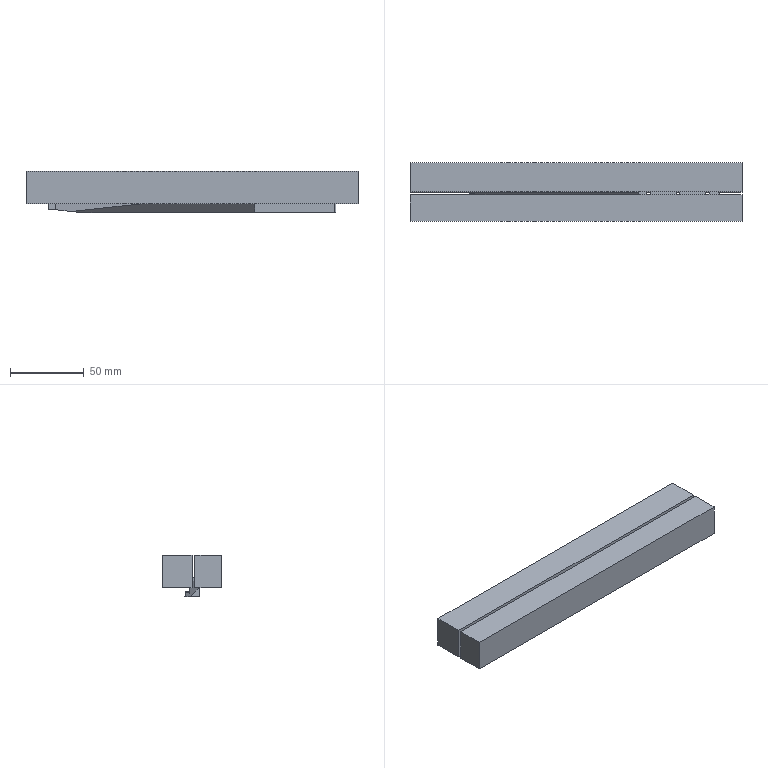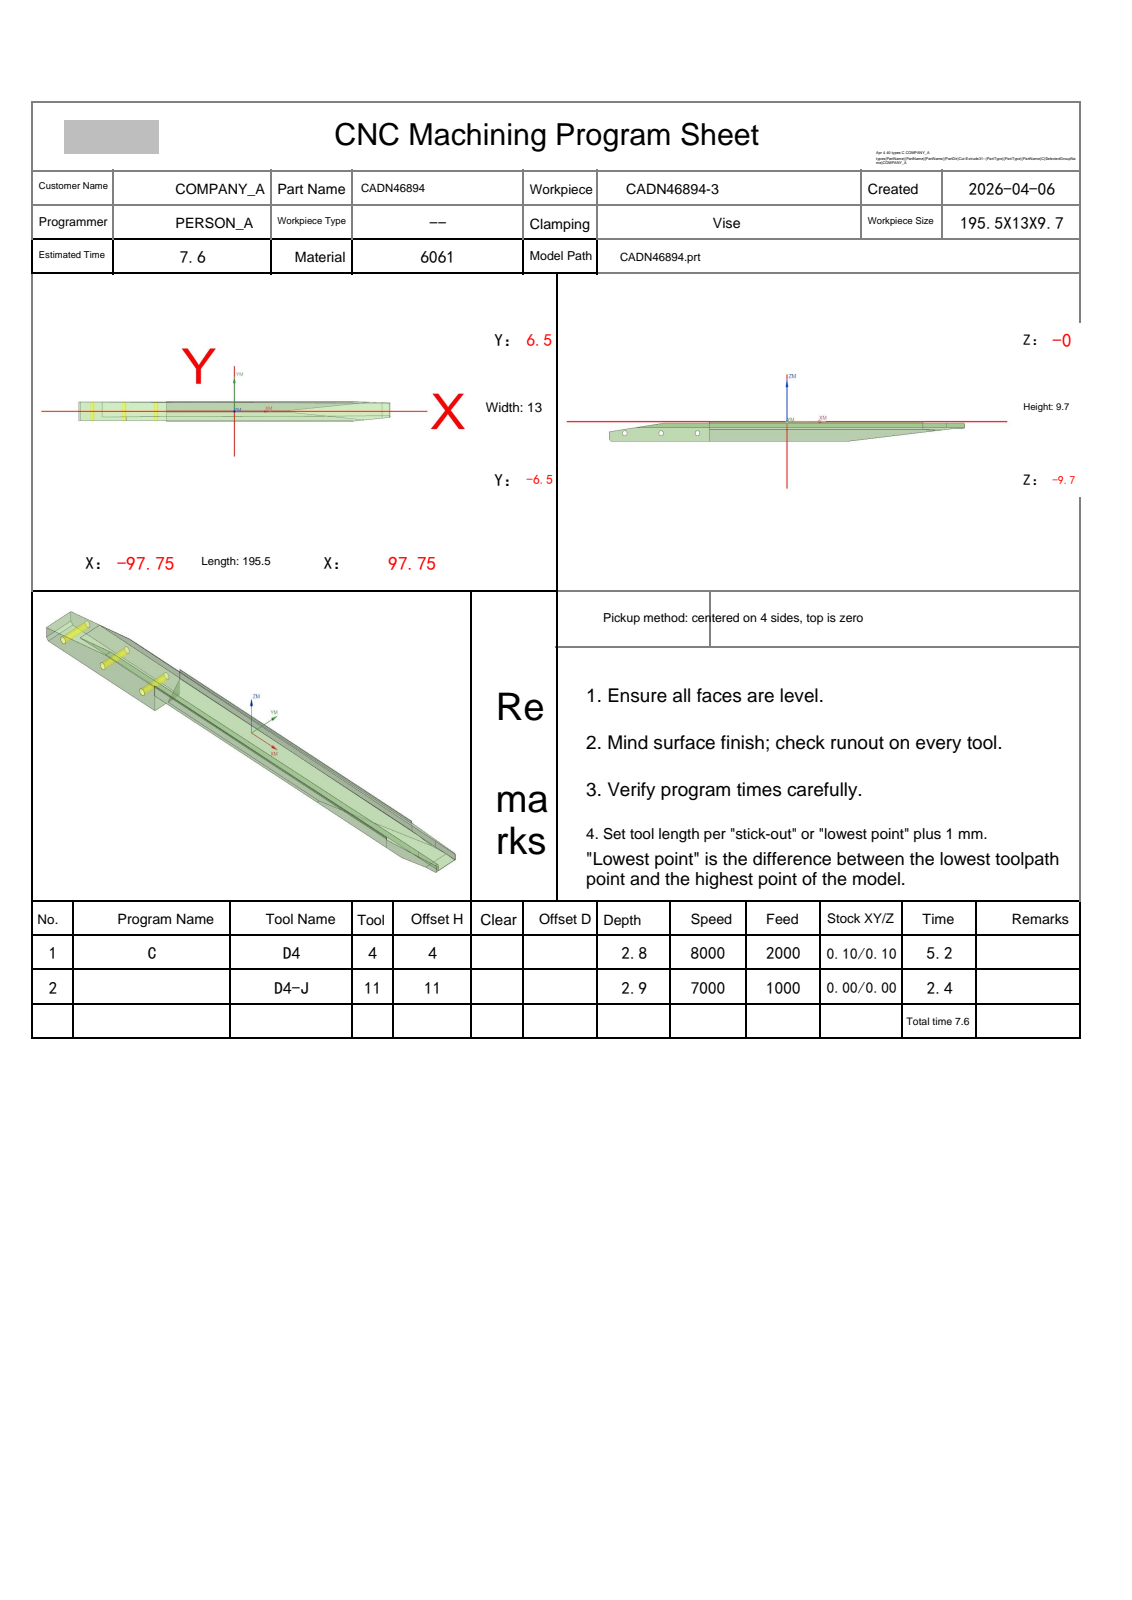NC program | NX | posted by the shop | part box 225.5 x 39.7 x 28 mm
Lines 1335 to 2406 of 20119:
N2 T17 M06
(D2-J  D=2. R=0. H=17 ce=0.00 di=0.00)
G00 G90 G54 X-18.314 Y-3.537 M03 S8000
G43 H17 Z44.
M08
Z-5.9
G01 X-18.313 Y-3.54 Z-5.93 F800.
X-18.309 Y-3.547 Z-5.958
X-18.302 Y-3.557 Z-5.982
X-18.293 Y-3.57 Z-6.004
X-18.282 Y-3.586 Z-6.023
X-18.268 Y-3.603 Z-6.04
X-18.253 Y-3.621 Z-6.054
X-18.235 Y-3.639 Z-6.066
X-18.215 Y-3.657 Z-6.076
X-18.193 Y-3.673 Z-6.084
X-18.169 Y-3.687 Z-6.09
X-18.143 Y-3.699 Z-6.095
X-18.115 Y-3.707 Z-6.098
X-18.086 Y-3.711 Z-6.099
X-18.055 Y-3.71 Z-6.1
X-5.108 Y-2.306
X-5. Y-2.3
X-3.
G02 X-.827 Y-2.797 I0.0 J-5.
X-1. Y-2.205 I.927 J.592
G01 Y-1.795
G02 X-.827 Y-1.203 I1.1 J0.0
G01 X-.847 Y-1.213
G02 X-3. Y-1.7 I-2.153 J4.513
G01 X-18.163
X-18.203 Y-1.718 Z-6.101
X-18.236 Y-1.767 Z-6.103
X-18.263 Y-1.843 Z-6.106
X-18.285 Y-1.939 Z-6.11
X-18.303 Y-2.05 Z-6.115
X-18.316 Y-2.17 Z-6.121
X-18.325 Y-2.293 Z-6.127
X-18.334 Y-2.578 Z-6.142
X-18.322 Y-2.858 Z-6.158
X-18.287 Y-3.14 Z-6.173
X-18.265 Y-3.262 Z-6.179
X-18.238 Y-3.379 Z-6.185
X-18.207 Y-3.487 Z-6.19
X-18.173 Y-3.58 Z-6.194
X-18.136 Y-3.652 Z-6.197
X-18.096 Y-3.697 Z-6.199
X-18.055 Y-3.71 Z-6.2
X-5.108 Y-2.306
X-5. Y-2.3
X-3.
G02 X-.827 Y-2.797 I0.0 J-5.
X-1. Y-2.205 I.927 J.592
G01 Y-1.795
G02 X-.827 Y-1.203 I1.1 J0.0
G01 X-.847 Y-1.213
G02 X-3. Y-1.7 I-2.153 J4.513
G01 X-18.163
X-18.203 Y-1.718 Z-6.201
X-18.236 Y-1.767 Z-6.203
X-18.263 Y-1.843 Z-6.206
X-18.285 Y-1.939 Z-6.21
X-18.303 Y-2.05 Z-6.215
X-18.316 Y-2.17 Z-6.221
X-18.325 Y-2.293 Z-6.227
X-18.334 Y-2.578 Z-6.242
X-18.322 Y-2.858 Z-6.258
X-18.287 Y-3.14 Z-6.273
X-18.265 Y-3.262 Z-6.279
X-18.238 Y-3.379 Z-6.285
X-18.207 Y-3.487 Z-6.29
X-18.173 Y-3.58 Z-6.294
X-18.136 Y-3.652 Z-6.297
X-18.096 Y-3.697 Z-6.299
X-18.055 Y-3.71 Z-6.3
X-5.108 Y-2.306
X-5. Y-2.3
X-3.
G02 X-.827 Y-2.797 I0.0 J-5.
X-1. Y-2.205 I.927 J.592
G01 Y-1.795
G02 X-.827 Y-1.203 I1.1 J0.0
G01 X-.847 Y-1.213
G02 X-3. Y-1.7 I-2.153 J4.513
G01 X-18.163
X-18.203 Y-1.718 Z-6.301
X-18.236 Y-1.767 Z-6.303
X-18.263 Y-1.843 Z-6.306
X-18.285 Y-1.939 Z-6.31
X-18.303 Y-2.05 Z-6.315
X-18.316 Y-2.17 Z-6.321
X-18.325 Y-2.293 Z-6.327
X-18.334 Y-2.578 Z-6.342
X-18.322 Y-2.858 Z-6.358
X-18.287 Y-3.14 Z-6.373
X-18.265 Y-3.262 Z-6.379
X-18.238 Y-3.379 Z-6.385
X-18.207 Y-3.487 Z-6.39
X-18.173 Y-3.58 Z-6.394
X-18.136 Y-3.652 Z-6.397
X-18.096 Y-3.697 Z-6.399
X-18.055 Y-3.71 Z-6.4
X-5.108 Y-2.306
X-5. Y-2.3
X-3.
G02 X-.827 Y-2.797 I0.0 J-5.
X-1. Y-2.205 I.927 J.592
G01 Y-1.795
G02 X-.827 Y-1.203 I1.1 J0.0
G01 X-.847 Y-1.213
G02 X-3. Y-1.7 I-2.153 J4.513
G01 X-18.163
X-18.203 Y-1.718 Z-6.401
X-18.236 Y-1.767 Z-6.403
X-18.263 Y-1.843 Z-6.406
X-18.285 Y-1.939 Z-6.41
X-18.303 Y-2.05 Z-6.415
X-18.316 Y-2.17 Z-6.421
X-18.325 Y-2.293 Z-6.427
X-18.334 Y-2.578 Z-6.442
X-18.322 Y-2.858 Z-6.458
X-18.287 Y-3.14 Z-6.473
X-18.265 Y-3.262 Z-6.479
X-18.238 Y-3.379 Z-6.485
X-18.207 Y-3.487 Z-6.49
X-18.173 Y-3.58 Z-6.494
X-18.136 Y-3.652 Z-6.497
X-18.096 Y-3.697 Z-6.499
X-18.055 Y-3.71 Z-6.5
X-5.108 Y-2.306
X-5. Y-2.3
X-3.
G02 X-.827 Y-2.797 I0.0 J-5.
X-1. Y-2.205 I.927 J.592
G01 Y-1.795
G02 X-.827 Y-1.203 I1.1 J0.0
G01 X-.847 Y-1.213
G02 X-3. Y-1.7 I-2.153 J4.513
G01 X-18.163
X-18.203 Y-1.718 Z-6.501
X-18.236 Y-1.767 Z-6.503
X-18.263 Y-1.843 Z-6.506
X-18.285 Y-1.939 Z-6.51
X-18.303 Y-2.05 Z-6.515
X-18.316 Y-2.17 Z-6.521
X-18.325 Y-2.293 Z-6.527
X-18.334 Y-2.578 Z-6.542
X-18.322 Y-2.858 Z-6.558
X-18.287 Y-3.14 Z-6.573
X-18.265 Y-3.262 Z-6.579
X-18.238 Y-3.379 Z-6.585
X-18.207 Y-3.487 Z-6.59
X-18.173 Y-3.58 Z-6.594
X-18.136 Y-3.652 Z-6.597
X-18.096 Y-3.697 Z-6.599
X-18.055 Y-3.71 Z-6.6
X-5.108 Y-2.306
X-5. Y-2.3
X-3.
G02 X-.827 Y-2.797 I0.0 J-5.
X-1. Y-2.205 I.927 J.592
G01 Y-1.795
G02 X-.827 Y-1.203 I1.1 J0.0
G01 X-.847 Y-1.213
G02 X-3. Y-1.7 I-2.153 J4.513
G01 X-18.163
X-18.203 Y-1.718 Z-6.601
X-18.236 Y-1.767 Z-6.603
X-18.263 Y-1.843 Z-6.606
X-18.285 Y-1.939 Z-6.61
X-18.303 Y-2.05 Z-6.615
X-18.316 Y-2.17 Z-6.621
X-18.325 Y-2.293 Z-6.627
X-18.334 Y-2.578 Z-6.642
X-18.322 Y-2.858 Z-6.658
X-18.287 Y-3.14 Z-6.673
X-18.265 Y-3.262 Z-6.679
X-18.238 Y-3.379 Z-6.685
X-18.207 Y-3.487 Z-6.69
X-18.173 Y-3.58 Z-6.694
X-18.136 Y-3.652 Z-6.697
X-18.096 Y-3.697 Z-6.699
X-18.055 Y-3.71 Z-6.7
X-5.108 Y-2.306
X-5. Y-2.3
X-3.
G02 X-.827 Y-2.797 I0.0 J-5.
X-1. Y-2.205 I.927 J.592
G01 Y-1.795
G02 X-.827 Y-1.203 I1.1 J0.0
G01 X-.847 Y-1.213
G02 X-3. Y-1.7 I-2.153 J4.513
G01 X-18.163
X-18.203 Y-1.718 Z-6.701
X-18.236 Y-1.767 Z-6.703
X-18.263 Y-1.843 Z-6.706
X-18.285 Y-1.939 Z-6.71
X-18.303 Y-2.05 Z-6.715
X-18.316 Y-2.17 Z-6.721
X-18.325 Y-2.293 Z-6.727
X-18.334 Y-2.578 Z-6.742
X-18.322 Y-2.858 Z-6.758
X-18.287 Y-3.14 Z-6.773
X-18.265 Y-3.262 Z-6.779
X-18.238 Y-3.379 Z-6.785
X-18.207 Y-3.487 Z-6.79
X-18.173 Y-3.58 Z-6.794
X-18.136 Y-3.652 Z-6.797
X-18.096 Y-3.697 Z-6.799
X-18.055 Y-3.71 Z-6.8
X-5.108 Y-2.306
X-5. Y-2.3
X-3.
G02 X-.827 Y-2.797 I0.0 J-5.
X-1. Y-2.205 I.927 J.592
G01 Y-1.795
G02 X-.827 Y-1.203 I1.1 J0.0
G01 X-.847 Y-1.213
G02 X-3. Y-1.7 I-2.153 J4.513
G01 X-18.163
X-18.203 Y-1.718 Z-6.801
X-18.236 Y-1.767 Z-6.803
X-18.263 Y-1.843 Z-6.806
X-18.285 Y-1.939 Z-6.81
X-18.303 Y-2.05 Z-6.815
X-18.316 Y-2.17 Z-6.821
X-18.325 Y-2.293 Z-6.827
X-18.334 Y-2.578 Z-6.842
X-18.322 Y-2.858 Z-6.858
X-18.287 Y-3.14 Z-6.873
X-18.265 Y-3.262 Z-6.879
X-18.238 Y-3.379 Z-6.885
X-18.207 Y-3.487 Z-6.89
X-18.173 Y-3.58 Z-6.894
X-18.136 Y-3.652 Z-6.897
X-18.096 Y-3.697 Z-6.899
X-18.055 Y-3.71 Z-6.9
X-5.108 Y-2.306
X-5. Y-2.3
X-3.
G02 X-.827 Y-2.797 I0.0 J-5.
X-1. Y-2.205 I.927 J.592
G01 Y-1.795
G02 X-.827 Y-1.203 I1.1 J0.0
G01 X-.847 Y-1.213
G02 X-3. Y-1.7 I-2.153 J4.513
G01 X-18.163
X-18.203 Y-1.718 Z-6.901
X-18.236 Y-1.767 Z-6.903
X-18.263 Y-1.843 Z-6.906
X-18.285 Y-1.939 Z-6.91
X-18.303 Y-2.05 Z-6.915
X-18.316 Y-2.17 Z-6.921
X-18.325 Y-2.293 Z-6.927
X-18.334 Y-2.578 Z-6.942
X-18.322 Y-2.858 Z-6.958
X-18.287 Y-3.14 Z-6.973
X-18.265 Y-3.262 Z-6.979
X-18.238 Y-3.379 Z-6.985
X-18.207 Y-3.487 Z-6.99
X-18.173 Y-3.58 Z-6.994
X-18.136 Y-3.652 Z-6.997
X-18.096 Y-3.697 Z-6.999
X-18.055 Y-3.71 Z-7.
X-5.108 Y-2.306
X-5. Y-2.3
X-3.
G02 X-.827 Y-2.797 I0.0 J-5.
X-1. Y-2.205 I.927 J.592
G01 Y-1.795
G02 X-.827 Y-1.203 I1.1 J0.0
G01 X-.847 Y-1.213
G02 X-3. Y-1.7 I-2.153 J4.513
G01 X-18.163
X-18.203 Y-1.718 Z-7.001
X-18.236 Y-1.767 Z-7.003
X-18.263 Y-1.843 Z-7.006
X-18.285 Y-1.939 Z-7.01
X-18.303 Y-2.05 Z-7.015
X-18.316 Y-2.17 Z-7.021
X-18.325 Y-2.293 Z-7.027
X-18.334 Y-2.578 Z-7.042
X-18.322 Y-2.858 Z-7.058
X-18.287 Y-3.14 Z-7.073
X-18.265 Y-3.262 Z-7.079
X-18.238 Y-3.379 Z-7.085
X-18.207 Y-3.487 Z-7.09
X-18.173 Y-3.58 Z-7.094
X-18.136 Y-3.652 Z-7.097
X-18.096 Y-3.697 Z-7.099
X-18.055 Y-3.71 Z-7.1
X-5.108 Y-2.306
X-5. Y-2.3
X-3.
G02 X-.827 Y-2.797 I0.0 J-5.
X-1. Y-2.205 I.927 J.592
G01 Y-1.795
G02 X-.827 Y-1.203 I1.1 J0.0
G01 X-.847 Y-1.213
G02 X-3. Y-1.7 I-2.153 J4.513
G01 X-18.163
X-18.203 Y-1.718 Z-7.101
X-18.236 Y-1.767 Z-7.103
X-18.263 Y-1.843 Z-7.106
X-18.285 Y-1.939 Z-7.11
X-18.303 Y-2.05 Z-7.115
X-18.316 Y-2.17 Z-7.121
X-18.325 Y-2.293 Z-7.127
X-18.334 Y-2.578 Z-7.142
X-18.322 Y-2.858 Z-7.158
X-18.287 Y-3.14 Z-7.173
X-18.265 Y-3.262 Z-7.179
X-18.238 Y-3.379 Z-7.185
X-18.207 Y-3.487 Z-7.19
X-18.173 Y-3.58 Z-7.194
X-18.136 Y-3.652 Z-7.197
X-18.096 Y-3.697 Z-7.199
X-18.055 Y-3.71 Z-7.2
X-5.108 Y-2.306
X-5. Y-2.3
X-3.
G02 X-.827 Y-2.797 I0.0 J-5.
X-1. Y-2.205 I.927 J.592
G01 Y-1.795
G02 X-.827 Y-1.203 I1.1 J0.0
G01 X-.847 Y-1.213
G02 X-3. Y-1.7 I-2.153 J4.513
G01 X-18.163
X-18.203 Y-1.718 Z-7.201
X-18.236 Y-1.767 Z-7.203
X-18.263 Y-1.843 Z-7.206
X-18.285 Y-1.939 Z-7.21
X-18.303 Y-2.05 Z-7.215
X-18.316 Y-2.17 Z-7.221
X-18.325 Y-2.293 Z-7.227
X-18.334 Y-2.578 Z-7.242
X-18.322 Y-2.858 Z-7.258
X-18.287 Y-3.14 Z-7.273
X-18.265 Y-3.262 Z-7.279
X-18.238 Y-3.379 Z-7.285
X-18.207 Y-3.487 Z-7.29
X-18.173 Y-3.58 Z-7.294
X-18.136 Y-3.652 Z-7.297
X-18.096 Y-3.697 Z-7.299
X-18.055 Y-3.71 Z-7.3
X-5.108 Y-2.306
X-5. Y-2.3
X-3.
G02 X-.827 Y-2.797 I0.0 J-5.
X-1. Y-2.205 I.927 J.592
G01 Y-1.795
G02 X-.827 Y-1.203 I1.1 J0.0
G01 X-.847 Y-1.213
G02 X-3. Y-1.7 I-2.153 J4.513
G01 X-18.163
X-18.203 Y-1.718 Z-7.301
X-18.236 Y-1.767 Z-7.303
X-18.263 Y-1.843 Z-7.306
X-18.285 Y-1.939 Z-7.31
X-18.303 Y-2.05 Z-7.315
X-18.316 Y-2.17 Z-7.321
X-18.325 Y-2.293 Z-7.327
X-18.334 Y-2.578 Z-7.342
X-18.322 Y-2.858 Z-7.358
X-18.287 Y-3.14 Z-7.373
X-18.265 Y-3.262 Z-7.379
X-18.238 Y-3.379 Z-7.385
X-18.207 Y-3.487 Z-7.39
X-18.173 Y-3.58 Z-7.394
X-18.136 Y-3.652 Z-7.397
X-18.096 Y-3.697 Z-7.399
X-18.055 Y-3.71 Z-7.4
X-5.108 Y-2.306
X-5. Y-2.3
X-3.
G02 X-.827 Y-2.797 I0.0 J-5.
X-1. Y-2.205 I.927 J.592
G01 Y-1.795
G02 X-.827 Y-1.203 I1.1 J0.0
G01 X-.847 Y-1.213
G02 X-3. Y-1.7 I-2.153 J4.513
G01 X-18.163
X-18.203 Y-1.718 Z-7.401
X-18.236 Y-1.767 Z-7.403
X-18.263 Y-1.843 Z-7.406
X-18.285 Y-1.939 Z-7.41
X-18.303 Y-2.05 Z-7.415
X-18.316 Y-2.17 Z-7.421
X-18.325 Y-2.293 Z-7.427
X-18.334 Y-2.578 Z-7.442
X-18.322 Y-2.858 Z-7.458
X-18.287 Y-3.14 Z-7.473
X-18.265 Y-3.262 Z-7.479
X-18.238 Y-3.379 Z-7.485
X-18.207 Y-3.487 Z-7.49
X-18.173 Y-3.58 Z-7.494
X-18.136 Y-3.652 Z-7.497
X-18.096 Y-3.697 Z-7.499
X-18.055 Y-3.71 Z-7.5
X-5.108 Y-2.306
X-5. Y-2.3
X-3.
G02 X-.827 Y-2.797 I0.0 J-5.
X-1. Y-2.205 I.927 J.592
G01 Y-1.795
G02 X-.827 Y-1.203 I1.1 J0.0
G01 X-.847 Y-1.213
G02 X-3. Y-1.7 I-2.153 J4.513
G01 X-18.163
X-18.203 Y-1.718 Z-7.501
X-18.236 Y-1.767 Z-7.503
X-18.263 Y-1.843 Z-7.506
X-18.285 Y-1.939 Z-7.51
X-18.303 Y-2.05 Z-7.515
X-18.316 Y-2.17 Z-7.521
X-18.325 Y-2.293 Z-7.527
X-18.334 Y-2.578 Z-7.542
X-18.322 Y-2.858 Z-7.558
X-18.287 Y-3.14 Z-7.573
X-18.265 Y-3.262 Z-7.579
X-18.238 Y-3.379 Z-7.585
X-18.207 Y-3.487 Z-7.59
X-18.173 Y-3.58 Z-7.594
X-18.136 Y-3.652 Z-7.597
X-18.096 Y-3.697 Z-7.599
X-18.055 Y-3.71 Z-7.6
X-5.108 Y-2.306
X-5. Y-2.3
X-3.
G02 X-.827 Y-2.797 I0.0 J-5.
X-1. Y-2.205 I.927 J.592
G01 Y-1.795
G02 X-.827 Y-1.203 I1.1 J0.0
G01 X-.847 Y-1.213
G02 X-3. Y-1.7 I-2.153 J4.513
G01 X-18.163
X-18.203 Y-1.718 Z-7.601
X-18.236 Y-1.767 Z-7.603
X-18.263 Y-1.843 Z-7.606
X-18.285 Y-1.939 Z-7.61
X-18.303 Y-2.05 Z-7.615
X-18.316 Y-2.17 Z-7.621
X-18.325 Y-2.293 Z-7.627
X-18.334 Y-2.578 Z-7.642
X-18.322 Y-2.858 Z-7.658
X-18.287 Y-3.14 Z-7.673
X-18.265 Y-3.262 Z-7.679
X-18.238 Y-3.379 Z-7.685
X-18.207 Y-3.487 Z-7.69
X-18.173 Y-3.58 Z-7.694
X-18.136 Y-3.652 Z-7.697
X-18.096 Y-3.697 Z-7.699
X-18.055 Y-3.71 Z-7.7
X-5.108 Y-2.306
X-5. Y-2.3
X-3.
G02 X-.827 Y-2.797 I0.0 J-5.
X-1. Y-2.205 I.927 J.592
G01 Y-1.795
G02 X-.827 Y-1.203 I1.1 J0.0
G01 X-.847 Y-1.213
G02 X-3. Y-1.7 I-2.153 J4.513
G01 X-18.163
X-18.203 Y-1.718 Z-7.701
X-18.236 Y-1.767 Z-7.703
X-18.263 Y-1.843 Z-7.706
X-18.285 Y-1.939 Z-7.71
X-18.303 Y-2.05 Z-7.715
X-18.316 Y-2.17 Z-7.721
X-18.325 Y-2.293 Z-7.727
X-18.334 Y-2.578 Z-7.742
X-18.322 Y-2.858 Z-7.758
X-18.287 Y-3.14 Z-7.773
X-18.265 Y-3.262 Z-7.779
X-18.238 Y-3.379 Z-7.785
X-18.207 Y-3.487 Z-7.79
X-18.173 Y-3.58 Z-7.794
X-18.136 Y-3.652 Z-7.797
X-18.096 Y-3.697 Z-7.799
X-18.055 Y-3.71 Z-7.8
X-5.108 Y-2.306
X-5. Y-2.3
X-3.
G02 X-.827 Y-2.797 I0.0 J-5.
X-1. Y-2.205 I.927 J.592
G01 Y-1.795
G02 X-.827 Y-1.203 I1.1 J0.0
G01 X-.847 Y-1.213
G02 X-3. Y-1.7 I-2.153 J4.513
G01 X-18.163
X-18.203 Y-1.718 Z-7.801
X-18.236 Y-1.767 Z-7.803
X-18.263 Y-1.843 Z-7.806
X-18.285 Y-1.939 Z-7.81
X-18.303 Y-2.05 Z-7.815
X-18.316 Y-2.17 Z-7.821
X-18.325 Y-2.293 Z-7.827
X-18.334 Y-2.578 Z-7.842
X-18.322 Y-2.858 Z-7.858
X-18.287 Y-3.14 Z-7.873
X-18.265 Y-3.262 Z-7.879
X-18.238 Y-3.379 Z-7.885
X-18.207 Y-3.487 Z-7.89
X-18.173 Y-3.58 Z-7.894
X-18.136 Y-3.652 Z-7.897
X-18.096 Y-3.697 Z-7.899
X-18.055 Y-3.71 Z-7.9
X-5.108 Y-2.306
X-5. Y-2.3
X-3.
G02 X-.827 Y-2.797 I0.0 J-5.
X-1. Y-2.205 I.927 J.592
G01 Y-1.795
G02 X-.827 Y-1.203 I1.1 J0.0
G01 X-.847 Y-1.213
G02 X-3. Y-1.7 I-2.153 J4.513
G01 X-18.163
X-18.203 Y-1.718 Z-7.901
X-18.236 Y-1.767 Z-7.903
X-18.263 Y-1.843 Z-7.906
X-18.285 Y-1.939 Z-7.91
X-18.303 Y-2.05 Z-7.915
X-18.316 Y-2.17 Z-7.921
X-18.325 Y-2.293 Z-7.927
X-18.334 Y-2.578 Z-7.942
X-18.322 Y-2.858 Z-7.958
X-18.287 Y-3.14 Z-7.973
X-18.265 Y-3.262 Z-7.979
X-18.238 Y-3.379 Z-7.985
X-18.207 Y-3.487 Z-7.99
X-18.173 Y-3.58 Z-7.994
X-18.136 Y-3.652 Z-7.997
X-18.096 Y-3.697 Z-7.999
X-18.055 Y-3.71 Z-8.
X-5.108 Y-2.306
X-5. Y-2.3
X-3.
G02 X-.827 Y-2.797 I0.0 J-5.
X-1. Y-2.205 I.927 J.592
G01 Y-1.795
G02 X-.827 Y-1.203 I1.1 J0.0
G01 X-.847 Y-1.213
G02 X-3. Y-1.7 I-2.153 J4.513
G01 X-18.163
X-18.203 Y-1.718 Z-8.001
X-18.236 Y-1.767 Z-8.003
X-18.263 Y-1.843 Z-8.006
X-18.285 Y-1.939 Z-8.01
X-18.303 Y-2.05 Z-8.015
X-18.316 Y-2.17 Z-8.021
X-18.325 Y-2.293 Z-8.027
X-18.334 Y-2.578 Z-8.042
X-18.322 Y-2.858 Z-8.058
X-18.287 Y-3.14 Z-8.073
X-18.265 Y-3.262 Z-8.079
X-18.238 Y-3.379 Z-8.085
X-18.207 Y-3.487 Z-8.09
X-18.173 Y-3.58 Z-8.094
X-18.136 Y-3.652 Z-8.097
X-18.096 Y-3.697 Z-8.099
X-18.055 Y-3.71 Z-8.1
X-5.108 Y-2.306
X-5. Y-2.3
X-3.
G02 X-.827 Y-2.797 I0.0 J-5.
X-1. Y-2.205 I.927 J.592
G01 Y-1.795
G02 X-.827 Y-1.203 I1.1 J0.0
G01 X-.847 Y-1.213
G02 X-3. Y-1.7 I-2.153 J4.513
G01 X-18.163
X-18.203 Y-1.718 Z-8.101
X-18.236 Y-1.767 Z-8.103
X-18.263 Y-1.843 Z-8.106
X-18.285 Y-1.939 Z-8.11
X-18.303 Y-2.05 Z-8.115
X-18.316 Y-2.17 Z-8.121
X-18.325 Y-2.293 Z-8.127
X-18.334 Y-2.578 Z-8.142
X-18.322 Y-2.858 Z-8.158
X-18.287 Y-3.14 Z-8.173
X-18.265 Y-3.262 Z-8.179
X-18.238 Y-3.379 Z-8.185
X-18.207 Y-3.487 Z-8.19
X-18.173 Y-3.58 Z-8.194
X-18.136 Y-3.652 Z-8.197
X-18.096 Y-3.697 Z-8.199
X-18.055 Y-3.71 Z-8.2
X-5.108 Y-2.306
X-5. Y-2.3
X-3.
G02 X-.827 Y-2.797 I0.0 J-5.
X-1. Y-2.205 I.927 J.592
G01 Y-1.795
G02 X-.827 Y-1.203 I1.1 J0.0
G01 X-.847 Y-1.213
G02 X-3. Y-1.7 I-2.153 J4.513
G01 X-18.163
X-18.203 Y-1.718 Z-8.201
X-18.236 Y-1.767 Z-8.203
X-18.263 Y-1.843 Z-8.206
X-18.285 Y-1.939 Z-8.21
X-18.303 Y-2.05 Z-8.215
X-18.316 Y-2.17 Z-8.221
X-18.325 Y-2.293 Z-8.227
X-18.334 Y-2.578 Z-8.242
X-18.322 Y-2.858 Z-8.258
X-18.287 Y-3.14 Z-8.273
X-18.265 Y-3.262 Z-8.279
X-18.238 Y-3.379 Z-8.285
X-18.207 Y-3.487 Z-8.29
X-18.173 Y-3.58 Z-8.294
X-18.136 Y-3.652 Z-8.297
X-18.096 Y-3.697 Z-8.299
X-18.055 Y-3.71 Z-8.3
X-5.108 Y-2.306
X-5. Y-2.3
X-3.
G02 X-.827 Y-2.797 I0.0 J-5.
X-1. Y-2.205 I.927 J.592
G01 Y-1.795
G02 X-.827 Y-1.203 I1.1 J0.0
G01 X-.847 Y-1.213
G02 X-3. Y-1.7 I-2.153 J4.513
G01 X-18.163
X-18.203 Y-1.718 Z-8.301
X-18.236 Y-1.767 Z-8.303
X-18.263 Y-1.843 Z-8.306
X-18.285 Y-1.939 Z-8.31
X-18.303 Y-2.05 Z-8.315
X-18.316 Y-2.17 Z-8.321
X-18.325 Y-2.293 Z-8.327
X-18.334 Y-2.578 Z-8.342
X-18.322 Y-2.858 Z-8.358
X-18.287 Y-3.14 Z-8.373
X-18.265 Y-3.262 Z-8.379
X-18.238 Y-3.379 Z-8.385
X-18.207 Y-3.487 Z-8.39
X-18.173 Y-3.58 Z-8.394
X-18.136 Y-3.652 Z-8.397
X-18.096 Y-3.697 Z-8.399
X-18.055 Y-3.71 Z-8.4
X-5.108 Y-2.306
X-5. Y-2.3
X-3.
G02 X-.827 Y-2.797 I0.0 J-5.
X-1. Y-2.205 I.927 J.592
G01 Y-1.795
G02 X-.827 Y-1.203 I1.1 J0.0
G01 X-.847 Y-1.213
G02 X-3. Y-1.7 I-2.153 J4.513
G01 X-18.163
X-18.203 Y-1.718 Z-8.401
X-18.236 Y-1.767 Z-8.403
X-18.263 Y-1.843 Z-8.406
X-18.285 Y-1.939 Z-8.41
X-18.303 Y-2.05 Z-8.415
X-18.316 Y-2.17 Z-8.421
X-18.325 Y-2.293 Z-8.427
X-18.334 Y-2.578 Z-8.442
X-18.322 Y-2.858 Z-8.458
X-18.287 Y-3.14 Z-8.473
X-18.265 Y-3.262 Z-8.479
X-18.238 Y-3.379 Z-8.485
X-18.207 Y-3.487 Z-8.49
X-18.173 Y-3.58 Z-8.494
X-18.136 Y-3.652 Z-8.497
X-18.096 Y-3.697 Z-8.499
X-18.055 Y-3.71 Z-8.5
X-5.108 Y-2.306
X-5. Y-2.3
X-3.
G02 X-.827 Y-2.797 I0.0 J-5.
X-1. Y-2.205 I.927 J.592
G01 Y-1.795
G02 X-.827 Y-1.203 I1.1 J0.0
G01 X-.847 Y-1.213
G02 X-3. Y-1.7 I-2.153 J4.513
G01 X-18.163
X-18.203 Y-1.718 Z-8.501
X-18.236 Y-1.767 Z-8.503
X-18.263 Y-1.843 Z-8.506
X-18.285 Y-1.939 Z-8.51
X-18.303 Y-2.05 Z-8.515
X-18.316 Y-2.17 Z-8.521
X-18.325 Y-2.293 Z-8.527
X-18.334 Y-2.578 Z-8.542
X-18.322 Y-2.858 Z-8.558
X-18.287 Y-3.14 Z-8.573
X-18.265 Y-3.262 Z-8.579
X-18.238 Y-3.379 Z-8.585
X-18.207 Y-3.487 Z-8.59
X-18.173 Y-3.58 Z-8.594
X-18.136 Y-3.652 Z-8.597
X-18.096 Y-3.697 Z-8.599
X-18.055 Y-3.71 Z-8.6
X-5.108 Y-2.306
X-5. Y-2.3
X-3.
G02 X-.827 Y-2.797 I0.0 J-5.
X-1. Y-2.205 I.927 J.592
G01 Y-1.795
G02 X-.827 Y-1.203 I1.1 J0.0
G01 X-.847 Y-1.213
G02 X-3. Y-1.7 I-2.153 J4.513
G01 X-18.163
X-18.203 Y-1.718 Z-8.601
X-18.236 Y-1.767 Z-8.603
X-18.263 Y-1.843 Z-8.606
X-18.285 Y-1.939 Z-8.61
X-18.303 Y-2.05 Z-8.615
X-18.316 Y-2.17 Z-8.621
X-18.325 Y-2.293 Z-8.627
X-18.334 Y-2.578 Z-8.642
X-18.322 Y-2.858 Z-8.658
X-18.287 Y-3.14 Z-8.673
X-18.265 Y-3.262 Z-8.679
X-18.238 Y-3.379 Z-8.685
X-18.207 Y-3.487 Z-8.69
X-18.173 Y-3.58 Z-8.694
X-18.136 Y-3.652 Z-8.697
X-18.096 Y-3.697 Z-8.699
X-18.055 Y-3.71 Z-8.7
X-5.108 Y-2.306
X-5. Y-2.3
X-3.
G02 X-.827 Y-2.797 I0.0 J-5.
X-1. Y-2.205 I.927 J.592
G01 Y-1.795
G02 X-.827 Y-1.203 I1.1 J0.0
G01 X-.847 Y-1.213
G02 X-3. Y-1.7 I-2.153 J4.513
G01 X-18.163
X-18.203 Y-1.718 Z-8.701
X-18.236 Y-1.767 Z-8.703
X-18.263 Y-1.843 Z-8.706
X-18.285 Y-1.939 Z-8.71
X-18.303 Y-2.05 Z-8.715
X-18.316 Y-2.17 Z-8.721
X-18.325 Y-2.293 Z-8.727
X-18.334 Y-2.578 Z-8.742
X-18.322 Y-2.858 Z-8.758
X-18.287 Y-3.14 Z-8.773
X-18.265 Y-3.262 Z-8.779
X-18.238 Y-3.379 Z-8.785
X-18.207 Y-3.487 Z-8.79
X-18.173 Y-3.58 Z-8.794
X-18.136 Y-3.652 Z-8.797
X-18.096 Y-3.697 Z-8.799
X-18.055 Y-3.71 Z-8.8
X-5.108 Y-2.306
X-5. Y-2.3
X-3.
G02 X-.827 Y-2.797 I0.0 J-5.
X-1. Y-2.205 I.927 J.592
G01 Y-1.795
G02 X-.827 Y-1.203 I1.1 J0.0
G01 X-.847 Y-1.213
G02 X-3. Y-1.7 I-2.153 J4.513
G01 X-18.163
X-18.203 Y-1.718 Z-8.801
X-18.236 Y-1.767 Z-8.803
X-18.263 Y-1.843 Z-8.806
X-18.285 Y-1.939 Z-8.81
X-18.303 Y-2.05 Z-8.815
X-18.316 Y-2.17 Z-8.821
X-18.325 Y-2.293 Z-8.827
X-18.334 Y-2.578 Z-8.842
X-18.322 Y-2.858 Z-8.858
X-18.287 Y-3.14 Z-8.873
X-18.265 Y-3.262 Z-8.879
X-18.238 Y-3.379 Z-8.885
X-18.207 Y-3.487 Z-8.89
X-18.173 Y-3.58 Z-8.894
X-18.136 Y-3.652 Z-8.897
X-18.096 Y-3.697 Z-8.899
X-18.055 Y-3.71 Z-8.9
X-5.108 Y-2.306
X-5. Y-2.3
X-3.
G02 X-.827 Y-2.797 I0.0 J-5.
X-1. Y-2.205 I.927 J.592
G01 Y-1.795
G02 X-.827 Y-1.203 I1.1 J0.0
G01 X-.847 Y-1.213
G02 X-3. Y-1.7 I-2.153 J4.513
G01 X-18.163
X-18.203 Y-1.718 Z-8.901
X-18.236 Y-1.767 Z-8.903
X-18.263 Y-1.843 Z-8.906
X-18.285 Y-1.939 Z-8.91
X-18.303 Y-2.05 Z-8.915
X-18.316 Y-2.17 Z-8.921
X-18.325 Y-2.293 Z-8.927
X-18.334 Y-2.578 Z-8.942
X-18.322 Y-2.858 Z-8.958
X-18.287 Y-3.14 Z-8.973
X-18.265 Y-3.262 Z-8.979
X-18.238 Y-3.379 Z-8.985
X-18.207 Y-3.487 Z-8.99
X-18.173 Y-3.58 Z-8.994
X-18.136 Y-3.652 Z-8.997
X-18.096 Y-3.697 Z-8.999
X-18.055 Y-3.71 Z-9.
X-5.108 Y-2.306
X-5. Y-2.3
X-3.
G02 X-.827 Y-2.797 I0.0 J-5.
X-1. Y-2.205 I.927 J.592
G01 Y-1.795
G02 X-.827 Y-1.203 I1.1 J0.0
G01 X-.847 Y-1.213
G02 X-3. Y-1.7 I-2.153 J4.513
G01 X-18.163
X-18.203 Y-1.718 Z-9.001
X-18.236 Y-1.767 Z-9.003
X-18.263 Y-1.843 Z-9.006
X-18.285 Y-1.939 Z-9.01
X-18.303 Y-2.05 Z-9.015
X-18.316 Y-2.17 Z-9.021
X-18.325 Y-2.293 Z-9.027
X-18.334 Y-2.578 Z-9.042
X-18.322 Y-2.858 Z-9.058
X-18.287 Y-3.14 Z-9.073
X-18.265 Y-3.262 Z-9.079
X-18.238 Y-3.379 Z-9.085
X-18.207 Y-3.487 Z-9.09
X-18.173 Y-3.58 Z-9.094
X-18.136 Y-3.652 Z-9.097
X-18.096 Y-3.697 Z-9.099
X-18.055 Y-3.71 Z-9.1
X-5.108 Y-2.306
X-5. Y-2.3
X-3.
G02 X-.827 Y-2.797 I0.0 J-5.
X-1. Y-2.205 I.927 J.592
G01 Y-1.795
G02 X-.827 Y-1.203 I1.1 J0.0
G01 X-.847 Y-1.213
G02 X-3. Y-1.7 I-2.153 J4.513
G01 X-18.163
X-18.203 Y-1.718 Z-9.101
X-18.236 Y-1.767 Z-9.103
X-18.263 Y-1.843 Z-9.106
X-18.285 Y-1.939 Z-9.11
X-18.303 Y-2.05 Z-9.115
X-18.316 Y-2.17 Z-9.121
X-18.325 Y-2.293 Z-9.127
X-18.334 Y-2.578 Z-9.142
X-18.322 Y-2.858 Z-9.158
X-18.287 Y-3.14 Z-9.173
X-18.265 Y-3.262 Z-9.179
X-18.238 Y-3.379 Z-9.185
X-18.207 Y-3.487 Z-9.19
X-18.173 Y-3.58 Z-9.194
X-18.136 Y-3.652 Z-9.197
X-18.096 Y-3.697 Z-9.199
X-18.055 Y-3.71 Z-9.2
X-5.108 Y-2.306
X-5. Y-2.3
X-3.
G02 X-.827 Y-2.797 I0.0 J-5.
X-1. Y-2.205 I.927 J.592
G01 Y-1.795
G02 X-.827 Y-1.203 I1.1 J0.0
X-3. Y-1.7 I-2.173 J4.503
G01 X-18.163
X-18.203 Y-1.718 Z-9.201
X-18.236 Y-1.767 Z-9.203
X-18.263 Y-1.843 Z-9.206
X-18.285 Y-1.939 Z-9.21
X-18.303 Y-2.05 Z-9.215
X-18.316 Y-2.17 Z-9.221
X-18.325 Y-2.293 Z-9.227
X-18.334 Y-2.578 Z-9.242
X-18.322 Y-2.858 Z-9.258
X-18.287 Y-3.14 Z-9.273
X-18.265 Y-3.262 Z-9.279
X-18.238 Y-3.379 Z-9.285
X-18.207 Y-3.487 Z-9.29
X-18.173 Y-3.58 Z-9.294
X-18.136 Y-3.652 Z-9.297
X-18.096 Y-3.697 Z-9.299
X-18.055 Y-3.71 Z-9.3
X-5.108 Y-2.306
X-5. Y-2.3
X-3.
G02 X-.827 Y-2.797 I0.0 J-5.
X-1. Y-2.205 I.927 J.592
G01 Y-1.795
G02 X-.827 Y-1.203 I1.1 J0.0
X-3. Y-1.7 I-2.173 J4.503
G01 X-18.163
X-18.203 Y-1.718 Z-9.301
X-18.236 Y-1.767 Z-9.303
X-18.263 Y-1.843 Z-9.306
X-18.285 Y-1.939 Z-9.31
X-18.303 Y-2.05 Z-9.315
X-18.316 Y-2.17 Z-9.321
X-18.325 Y-2.293 Z-9.327
X-18.334 Y-2.578 Z-9.342
X-18.322 Y-2.858 Z-9.358
X-18.287 Y-3.14 Z-9.373
X-18.265 Y-3.262 Z-9.379
X-18.238 Y-3.379 Z-9.385
X-18.207 Y-3.487 Z-9.39
X-18.173 Y-3.58 Z-9.394
X-18.136 Y-3.652 Z-9.397
X-18.096 Y-3.697 Z-9.399
X-18.055 Y-3.71 Z-9.4
X-5.108 Y-2.306
X-5. Y-2.3
X-3.
G02 X-.827 Y-2.797 I0.0 J-5.
X-1. Y-2.205 I.927 J.592
G01 Y-1.795
G02 X-.827 Y-1.203 I1.1 J0.0
X-3. Y-1.7 I-2.173 J4.503
G01 X-18.163
X-18.203 Y-1.718 Z-9.401
X-18.236 Y-1.767 Z-9.403
X-18.263 Y-1.843 Z-9.406
X-18.285 Y-1.939 Z-9.41
X-18.303 Y-2.05 Z-9.415
X-18.316 Y-2.17 Z-9.421
X-18.325 Y-2.293 Z-9.427
X-18.334 Y-2.578 Z-9.442
X-18.322 Y-2.858 Z-9.458
X-18.287 Y-3.14 Z-9.473
X-18.265 Y-3.262 Z-9.479
X-18.238 Y-3.379 Z-9.485
X-18.207 Y-3.487 Z-9.49
X-18.173 Y-3.58 Z-9.494
X-18.136 Y-3.652 Z-9.497
X-18.096 Y-3.697 Z-9.499
X-18.055 Y-3.71 Z-9.5
X-5.108 Y-2.306
X-5. Y-2.3
X-3.
G02 X-.827 Y-2.797 I0.0 J-5.
X-1. Y-2.205 I.927 J.592
G01 Y-1.795
G02 X-.827 Y-1.203 I1.1 J0.0
X-3. Y-1.7 I-2.173 J4.503
G01 X-18.163
X-18.203 Y-1.718 Z-9.501
X-18.236 Y-1.767 Z-9.503
X-18.263 Y-1.843 Z-9.506
X-18.285 Y-1.939 Z-9.51
X-18.303 Y-2.05 Z-9.515
X-18.316 Y-2.17 Z-9.521
X-18.325 Y-2.293 Z-9.527
X-18.334 Y-2.578 Z-9.542
X-18.322 Y-2.858 Z-9.558
X-18.287 Y-3.14 Z-9.573
X-18.265 Y-3.262 Z-9.579
X-18.238 Y-3.379 Z-9.585
X-18.207 Y-3.487 Z-9.59
X-18.173 Y-3.58 Z-9.594
X-18.136 Y-3.652 Z-9.597
X-18.096 Y-3.697 Z-9.599
X-18.055 Y-3.71 Z-9.6
X-5.108 Y-2.306
X-5. Y-2.3
X-3.
G02 X-.827 Y-2.797 I0.0 J-5.
X-1. Y-2.205 I.927 J.592
G01 Y-1.795
G02 X-.827 Y-1.203 I1.1 J0.0
X-3. Y-1.7 I-2.173 J4.503
G01 X-18.163
X-18.203 Y-1.718 Z-9.601
X-18.236 Y-1.767 Z-9.603
X-18.263 Y-1.843 Z-9.606
X-18.285 Y-1.939 Z-9.61
X-18.303 Y-2.05 Z-9.615
X-18.316 Y-2.17 Z-9.621
X-18.325 Y-2.293 Z-9.627
X-18.334 Y-2.578 Z-9.642
X-18.322 Y-2.858 Z-9.658
X-18.287 Y-3.14 Z-9.673
X-18.265 Y-3.262 Z-9.679
X-18.238 Y-3.379 Z-9.685
X-18.207 Y-3.487 Z-9.69
X-18.173 Y-3.58 Z-9.694
X-18.136 Y-3.652 Z-9.697
X-18.096 Y-3.697 Z-9.699
X-18.055 Y-3.71 Z-9.7
X-5.108 Y-2.306
X-5. Y-2.3
X-3.
G02 X-.827 Y-2.797 I0.0 J-5.
X-1. Y-2.205 I.927 J.592
G01 Y-1.795
G02 X-.827 Y-1.203 I1.1 J0.0
X-3. Y-1.7 I-2.173 J4.503
G01 X-18.163
X-18.203 Y-1.718 Z-9.701
X-18.236 Y-1.767 Z-9.703
X-18.263 Y-1.843 Z-9.706
X-18.285 Y-1.939 Z-9.71
X-18.303 Y-2.05 Z-9.715
X-18.316 Y-2.17 Z-9.721
X-18.325 Y-2.293 Z-9.727
X-18.334 Y-2.578 Z-9.742
X-18.322 Y-2.858 Z-9.758
X-18.287 Y-3.14 Z-9.773
X-18.265 Y-3.262 Z-9.779
X-18.238 Y-3.379 Z-9.785
X-18.207 Y-3.487 Z-9.79
X-18.173 Y-3.58 Z-9.794
X-18.136 Y-3.652 Z-9.797
X-18.096 Y-3.697 Z-9.799
X-18.055 Y-3.71 Z-9.8
X-5.108 Y-2.306
X-5. Y-2.3
X-3.
G02 X-.827 Y-2.797 I0.0 J-5.
X-1. Y-2.205 I.927 J.592
G01 Y-1.795
G02 X-.827 Y-1.203 I1.1 J0.0
X-3. Y-1.7 I-2.173 J4.503
G01 X-18.163
X-18.203 Y-1.718 Z-9.801
X-18.236 Y-1.767 Z-9.803
X-18.263 Y-1.843 Z-9.806
X-18.285 Y-1.939 Z-9.81
X-18.303 Y-2.05 Z-9.815
X-18.316 Y-2.17 Z-9.821
X-18.325 Y-2.293 Z-9.827
X-18.334 Y-2.578 Z-9.842
X-18.322 Y-2.858 Z-9.858
X-18.287 Y-3.14 Z-9.873
X-18.265 Y-3.262 Z-9.879
X-18.238 Y-3.379 Z-9.885
X-18.207 Y-3.487 Z-9.89
X-18.173 Y-3.58 Z-9.894
X-18.136 Y-3.652 Z-9.897
X-18.096 Y-3.697 Z-9.899
X-18.055 Y-3.71 Z-9.9
X-5.108 Y-2.306
X-5. Y-2.3
X-3.
G02 X-.827 Y-2.797 I0.0 J-5.
X-1. Y-2.205 I.927 J.592
G01 Y-1.795
G02 X-.827 Y-1.203 I1.1 J0.0
X-3. Y-1.7 I-2.173 J4.503
G01 X-18.163
X-18.203 Y-1.718 Z-9.901
X-18.236 Y-1.767 Z-9.903
X-18.263 Y-1.843 Z-9.906
X-18.285 Y-1.939 Z-9.91
X-18.303 Y-2.05 Z-9.915
X-18.316 Y-2.17 Z-9.921
X-18.325 Y-2.293 Z-9.927
X-18.334 Y-2.578 Z-9.942
X-18.322 Y-2.858 Z-9.958
X-18.287 Y-3.14 Z-9.973
X-18.265 Y-3.262 Z-9.979
X-18.238 Y-3.379 Z-9.985
X-18.207 Y-3.487 Z-9.99
X-18.173 Y-3.58 Z-9.994
X-18.136 Y-3.652 Z-9.997
X-18.096 Y-3.697 Z-9.999
X-18.055 Y-3.71 Z-10.
X-5.108 Y-2.306
X-5. Y-2.3
X-3.
G02 X-.827 Y-2.797 I0.0 J-5.
X-1. Y-2.205 I.927 J.592
G01 Y-1.795